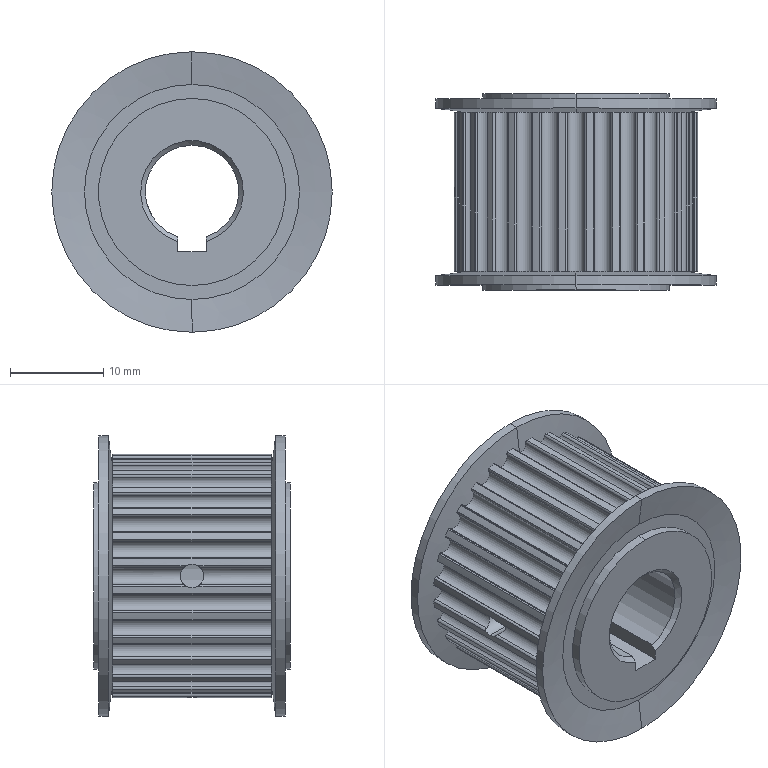Part | STEP file | 1 solid | 175 faces | box 30 x 21 x 30 mm | volume 8430 mm3 | cylinder 155 | cone 11 | plane 9 | commonest cylinder face diameters 0.665 x68 1.8 x45 26.11 x28 2.5 x4 20 x4 30 x4